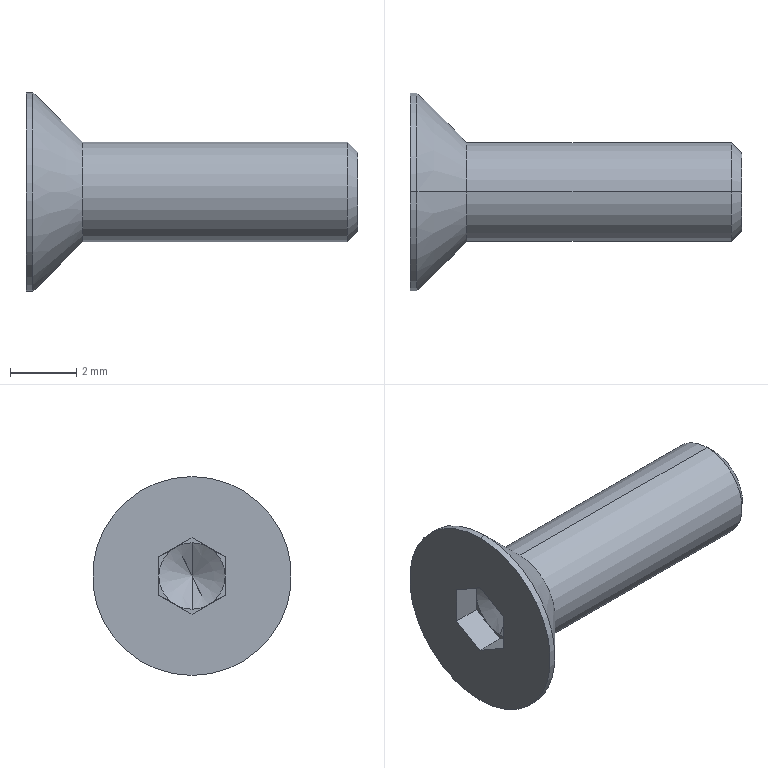Part | NX | features BREP 1 | 1 solid | 24 faces | box 10 x 6 x 6 mm | volume 85.103 mm3 | plane 14 | cone 6 | cylinder 4 | commonest cylinder face diameters 3 x2 6 x2
STEP:
#1=CARTESIAN_POINT('',(1.427,0.,0.));
#2=VERTEX_POINT('',#1);
#3=CARTESIAN_POINT('',(0.85,0.,1.));
#4=VERTEX_POINT('',#3);
#5=CARTESIAN_POINT('',(0.85,0.,1.));
#6=DIRECTION('',(-0.5,0.,0.866));
#7=VECTOR('',#6,1000.);
#8=LINE('',#5,#7);
#9=EDGE_CURVE('',#2,#4,#8,.T.);
#10=ORIENTED_EDGE('',*,*,#9,.F.);
#11=CARTESIAN_POINT('',(0.85,0.,-1.));
#12=VERTEX_POINT('',#11);
#13=CARTESIAN_POINT('',(0.85,0.,-1.));
#14=DIRECTION('',(-0.5,0.,-0.866));
#15=VECTOR('',#14,1000.);
#16=LINE('',#13,#15);
#17=EDGE_CURVE('',#2,#12,#16,.T.);
#18=ORIENTED_EDGE('',*,*,#17,.T.);
#19=CARTESIAN_POINT('',(0.85,-0.5,-0.866));
#20=VERTEX_POINT('',#19);
#21=CARTESIAN_POINT('',(0.85,0.,0.));
#22=DIRECTION('',(-1.,0.,0.));
#23=DIRECTION('',(0.,0.,1.));
#24=AXIS2_PLACEMENT_3D('',#21,#22,#23);
#25=CIRCLE('',#24,1.);
#26=EDGE_CURVE('',#12,#20,#25,.T.);
#27=ORIENTED_EDGE('',*,*,#26,.T.);
#28=CARTESIAN_POINT('',(0.85,-1.,0.));
#29=VERTEX_POINT('',#28);
#30=CARTESIAN_POINT('',(0.85,0.,0.));
#31=DIRECTION('',(-1.,0.,0.));
#32=DIRECTION('',(0.,0.,1.));
#33=AXIS2_PLACEMENT_3D('',#30,#31,#32);
#34=CIRCLE('',#33,1.);
#35=EDGE_CURVE('',#20,#29,#34,.T.);
#36=ORIENTED_EDGE('',*,*,#35,.T.);
#37=CARTESIAN_POINT('',(0.85,-0.5,0.866));
#38=VERTEX_POINT('',#37);
#39=CARTESIAN_POINT('',(0.85,0.,0.));
#40=DIRECTION('',(-1.,0.,0.));
#41=DIRECTION('',(0.,0.,1.));
#42=AXIS2_PLACEMENT_3D('',#39,#40,#41);
#43=CIRCLE('',#42,1.);
#44=EDGE_CURVE('',#29,#38,#43,.T.);
#45=ORIENTED_EDGE('',*,*,#44,.T.);
#46=CARTESIAN_POINT('',(0.85,0.,0.));
#47=DIRECTION('',(-1.,0.,0.));
#48=DIRECTION('',(0.,0.,1.));
#49=AXIS2_PLACEMENT_3D('',#46,#47,#48);
#50=CIRCLE('',#49,1.);
#51=EDGE_CURVE('',#38,#4,#50,.T.);
#52=ORIENTED_EDGE('',*,*,#51,.T.);
#53=EDGE_LOOP('',(#10,#18,#27,#36,#45,#52));
#54=FACE_BOUND('',#53,.T.);
#55=CARTESIAN_POINT('',(0.85,0.,0.));
#56=DIRECTION('',(-1.,0.,0.));
#57=DIRECTION('',(0.,0.,-1.));
#58=AXIS2_PLACEMENT_3D('',#55,#56,#57);
#59=CONICAL_SURFACE('',#58,1.,1.047);
#60=ADVANCED_FACE('',(#54),#59,.F.);
#61=CARTESIAN_POINT('',(10.,0.,1.194));
#62=VERTEX_POINT('',#61);
#63=CARTESIAN_POINT('',(10.,0.,-1.194));
#64=VERTEX_POINT('',#63);
#65=CARTESIAN_POINT('',(10.,0.,0.));
#66=DIRECTION('',(-1.,0.,0.));
#67=DIRECTION('',(0.,0.,1.));
#68=AXIS2_PLACEMENT_3D('',#65,#66,#67);
#69=CIRCLE('',#68,1.194);
#70=EDGE_CURVE('',#62,#64,#69,.T.);
#71=ORIENTED_EDGE('',*,*,#70,.T.);
#72=CARTESIAN_POINT('',(9.694,0.,-1.5));
#73=VERTEX_POINT('',#72);
#74=CARTESIAN_POINT('',(10.,0.,-1.194));
#75=DIRECTION('',(-0.7071,0.,-0.7071));
#76=VECTOR('',#75,1000.);
#77=LINE('',#74,#76);
#78=EDGE_CURVE('',#64,#73,#77,.T.);
#79=ORIENTED_EDGE('',*,*,#78,.T.);
#80=CARTESIAN_POINT('',(9.694,0.,1.5));
#81=VERTEX_POINT('',#80);
#82=CARTESIAN_POINT('',(9.694,0.,0.));
#83=DIRECTION('',(-1.,0.,0.));
#84=DIRECTION('',(0.,0.,1.));
#85=AXIS2_PLACEMENT_3D('',#82,#83,#84);
#86=CIRCLE('',#85,1.5);
#87=EDGE_CURVE('',#81,#73,#86,.T.);
#88=ORIENTED_EDGE('',*,*,#87,.F.);
#89=CARTESIAN_POINT('',(10.,0.,1.194));
#90=DIRECTION('',(-0.7071,0.,0.7071));
#91=VECTOR('',#90,1000.);
#92=LINE('',#89,#91);
#93=EDGE_CURVE('',#62,#81,#92,.T.);
#94=ORIENTED_EDGE('',*,*,#93,.F.);
#95=EDGE_LOOP('',(#71,#79,#88,#94));
#96=FACE_BOUND('',#95,.T.);
#97=CARTESIAN_POINT('',(10.,0.,0.));
#98=DIRECTION('',(-1.,0.,0.));
#99=DIRECTION('',(0.,0.,-1.));
#100=AXIS2_PLACEMENT_3D('',#97,#98,#99);
#101=CONICAL_SURFACE('',#100,1.194,0.7854);
#102=ADVANCED_FACE('',(#96),#101,.T.);
#103=ORIENTED_EDGE('',*,*,#87,.T.);
#104=CARTESIAN_POINT('',(1.7,0.,-1.5));
#105=VERTEX_POINT('',#104);
#106=CARTESIAN_POINT('',(10.,0.,-1.5));
#107=DIRECTION('',(-1.,0.,0.));
#108=VECTOR('',#107,1000.);
#109=LINE('',#106,#108);
#110=EDGE_CURVE('',#73,#105,#109,.T.);
#111=ORIENTED_EDGE('',*,*,#110,.T.);
#112=CARTESIAN_POINT('',(1.7,0.,1.5));
#113=VERTEX_POINT('',#112);
#114=CARTESIAN_POINT('',(1.7,0.,0.));
#115=DIRECTION('',(-1.,0.,0.));
#116=DIRECTION('',(0.,0.,1.));
#117=AXIS2_PLACEMENT_3D('',#114,#115,#116);
#118=CIRCLE('',#117,1.5);
#119=EDGE_CURVE('',#113,#105,#118,.T.);
#120=ORIENTED_EDGE('',*,*,#119,.F.);
#121=CARTESIAN_POINT('',(10.,0.,1.5));
#122=DIRECTION('',(-1.,0.,0.));
#123=VECTOR('',#122,1000.);
#124=LINE('',#121,#123);
#125=EDGE_CURVE('',#81,#113,#124,.T.);
#126=ORIENTED_EDGE('',*,*,#125,.F.);
#127=EDGE_LOOP('',(#103,#111,#120,#126));
#128=FACE_BOUND('',#127,.T.);
#129=CARTESIAN_POINT('',(10.,0.,0.));
#130=DIRECTION('',(-1.,0.,0.));
#131=DIRECTION('',(0.,0.,-1.));
#132=AXIS2_PLACEMENT_3D('',#129,#130,#131);
#133=CYLINDRICAL_SURFACE('',#132,1.5);
#134=ADVANCED_FACE('',(#128),#133,.T.);
#135=ORIENTED_EDGE('',*,*,#119,.T.);
#136=CARTESIAN_POINT('',(0.2,0.,-3.));
#137=VERTEX_POINT('',#136);
#138=CARTESIAN_POINT('',(1.7,0.,-1.5));
#139=DIRECTION('',(-0.7071,0.,-0.7071));
#140=VECTOR('',#139,1000.);
#141=LINE('',#138,#140);
#142=EDGE_CURVE('',#105,#137,#141,.T.);
#143=ORIENTED_EDGE('',*,*,#142,.T.);
#144=CARTESIAN_POINT('',(0.2,0.,3.));
#145=VERTEX_POINT('',#144);
#146=CARTESIAN_POINT('',(0.2,0.,0.));
#147=DIRECTION('',(-1.,0.,0.));
#148=DIRECTION('',(0.,0.,1.));
#149=AXIS2_PLACEMENT_3D('',#146,#147,#148);
#150=CIRCLE('',#149,3.);
#151=EDGE_CURVE('',#145,#137,#150,.T.);
#152=ORIENTED_EDGE('',*,*,#151,.F.);
#153=CARTESIAN_POINT('',(1.7,0.,1.5));
#154=DIRECTION('',(-0.7071,0.,0.7071));
#155=VECTOR('',#154,1000.);
#156=LINE('',#153,#155);
#157=EDGE_CURVE('',#113,#145,#156,.T.);
#158=ORIENTED_EDGE('',*,*,#157,.F.);
#159=EDGE_LOOP('',(#135,#143,#152,#158));
#160=FACE_BOUND('',#159,.T.);
#161=CARTESIAN_POINT('',(1.7,0.,0.));
#162=DIRECTION('',(-1.,0.,0.));
#163=DIRECTION('',(0.,0.,-1.));
#164=AXIS2_PLACEMENT_3D('',#161,#162,#163);
#165=CONICAL_SURFACE('',#164,1.5,0.7854);
#166=ADVANCED_FACE('',(#160),#165,.T.);
#167=ORIENTED_EDGE('',*,*,#151,.T.);
#168=CARTESIAN_POINT('',(0.,0.,-3.));
#169=VERTEX_POINT('',#168);
#170=CARTESIAN_POINT('',(10.,0.,-3.));
#171=DIRECTION('',(-1.,0.,0.));
#172=VECTOR('',#171,1000.);
#173=LINE('',#170,#172);
#174=EDGE_CURVE('',#137,#169,#173,.T.);
#175=ORIENTED_EDGE('',*,*,#174,.T.);
#176=CARTESIAN_POINT('',(0.,0.,3.));
#177=VERTEX_POINT('',#176);
#178=CARTESIAN_POINT('',(0.,0.,0.));
#179=DIRECTION('',(-1.,0.,0.));
#180=DIRECTION('',(0.,0.,1.));
#181=AXIS2_PLACEMENT_3D('',#178,#179,#180);
#182=CIRCLE('',#181,3.);
#183=EDGE_CURVE('',#177,#169,#182,.T.);
#184=ORIENTED_EDGE('',*,*,#183,.F.);
#185=CARTESIAN_POINT('',(10.,0.,3.));
#186=DIRECTION('',(-1.,0.,0.));
#187=VECTOR('',#186,1000.);
#188=LINE('',#185,#187);
#189=EDGE_CURVE('',#145,#177,#188,.T.);
#190=ORIENTED_EDGE('',*,*,#189,.F.);
#191=EDGE_LOOP('',(#167,#175,#184,#190));
#192=FACE_BOUND('',#191,.T.);
#193=CARTESIAN_POINT('',(10.,0.,0.));
#194=DIRECTION('',(-1.,0.,0.));
#195=DIRECTION('',(0.,0.,-1.));
#196=AXIS2_PLACEMENT_3D('',#193,#194,#195);
#197=CYLINDRICAL_SURFACE('',#196,3.);
#198=ADVANCED_FACE('',(#192),#197,.T.);
#199=CARTESIAN_POINT('',(0.,0.,1.155));
#200=VERTEX_POINT('',#199);
#201=CARTESIAN_POINT('',(0.,-1.,0.5774));
#202=VERTEX_POINT('',#201);
#203=CARTESIAN_POINT('',(0.,0.25,1.299));
#204=DIRECTION('',(0.,-0.866,-0.5));
#205=VECTOR('',#204,1000.);
#206=LINE('',#203,#205);
#207=EDGE_CURVE('',#200,#202,#206,.T.);
#208=ORIENTED_EDGE('',*,*,#207,.T.);
#209=CARTESIAN_POINT('',(0.,-1.,-0.5774));
#210=VERTEX_POINT('',#209);
#211=CARTESIAN_POINT('',(0.,-1.,0.));
#212=DIRECTION('',(0.,0.,-1.));
#213=VECTOR('',#212,1000.);
#214=LINE('',#211,#213);
#215=EDGE_CURVE('',#202,#210,#214,.T.);
#216=ORIENTED_EDGE('',*,*,#215,.T.);
#217=CARTESIAN_POINT('',(0.,0.,-1.155));
#218=VERTEX_POINT('',#217);
#219=CARTESIAN_POINT('',(0.,0.25,-1.299));
#220=DIRECTION('',(0.,0.866,-0.5));
#221=VECTOR('',#220,1000.);
#222=LINE('',#219,#221);
#223=EDGE_CURVE('',#210,#218,#222,.T.);
#224=ORIENTED_EDGE('',*,*,#223,.T.);
#225=CARTESIAN_POINT('',(0.,1.,-0.5774));
#226=VERTEX_POINT('',#225);
#227=CARTESIAN_POINT('',(0.,1.25,-0.433));
#228=DIRECTION('',(0.,0.866,0.5));
#229=VECTOR('',#228,1000.);
#230=LINE('',#227,#229);
#231=EDGE_CURVE('',#218,#226,#230,.T.);
#232=ORIENTED_EDGE('',*,*,#231,.T.);
#233=CARTESIAN_POINT('',(0.,1.,0.5774));
#234=VERTEX_POINT('',#233);
#235=CARTESIAN_POINT('',(0.,1.,0.));
#236=DIRECTION('',(0.,0.,1.));
#237=VECTOR('',#236,1000.);
#238=LINE('',#235,#237);
#239=EDGE_CURVE('',#226,#234,#238,.T.);
#240=ORIENTED_EDGE('',*,*,#239,.T.);
#241=CARTESIAN_POINT('',(0.,1.25,0.433));
#242=DIRECTION('',(0.,-0.866,0.5));
#243=VECTOR('',#242,1000.);
#244=LINE('',#241,#243);
#245=EDGE_CURVE('',#234,#200,#244,.T.);
#246=ORIENTED_EDGE('',*,*,#245,.T.);
#247=EDGE_LOOP('',(#208,#216,#224,#232,#240,#246));
#248=FACE_BOUND('',#247,.T.);
#249=ORIENTED_EDGE('',*,*,#183,.T.);
#250=CARTESIAN_POINT('',(0.,0.,0.));
#251=DIRECTION('',(-1.,0.,0.));
#252=DIRECTION('',(0.,0.,1.));
#253=AXIS2_PLACEMENT_3D('',#250,#251,#252);
#254=CIRCLE('',#253,3.);
#255=EDGE_CURVE('',#169,#177,#254,.T.);
#256=ORIENTED_EDGE('',*,*,#255,.T.);
#257=EDGE_LOOP('',(#249,#256));
#258=FACE_BOUND('',#257,.T.);
#259=CARTESIAN_POINT('',(0.,1.,0.));
#260=DIRECTION('',(1.,0.,0.));
#261=DIRECTION('',(0.,0.,1.));
#262=AXIS2_PLACEMENT_3D('',#259,#260,#261);
#263=PLANE('',#262);
#264=ADVANCED_FACE('',(#248,#258),#263,.F.);
#265=ORIENTED_EDGE('',*,*,#174,.F.);
#266=CARTESIAN_POINT('',(0.2,0.,0.));
#267=DIRECTION('',(-1.,0.,0.));
#268=DIRECTION('',(0.,0.,1.));
#269=AXIS2_PLACEMENT_3D('',#266,#267,#268);
#270=CIRCLE('',#269,3.);
#271=EDGE_CURVE('',#137,#145,#270,.T.);
#272=ORIENTED_EDGE('',*,*,#271,.T.);
#273=ORIENTED_EDGE('',*,*,#189,.T.);
#274=ORIENTED_EDGE('',*,*,#255,.F.);
#275=EDGE_LOOP('',(#265,#272,#273,#274));
#276=FACE_BOUND('',#275,.T.);
#277=CARTESIAN_POINT('',(10.,0.,0.));
#278=DIRECTION('',(-1.,0.,0.));
#279=DIRECTION('',(0.,0.,-1.));
#280=AXIS2_PLACEMENT_3D('',#277,#278,#279);
#281=CYLINDRICAL_SURFACE('',#280,3.);
#282=ADVANCED_FACE('',(#276),#281,.T.);
#283=ORIENTED_EDGE('',*,*,#142,.F.);
#284=CARTESIAN_POINT('',(1.7,0.,0.));
#285=DIRECTION('',(-1.,0.,0.));
#286=DIRECTION('',(0.,0.,1.));
#287=AXIS2_PLACEMENT_3D('',#284,#285,#286);
#288=CIRCLE('',#287,1.5);
#289=EDGE_CURVE('',#105,#113,#288,.T.);
#290=ORIENTED_EDGE('',*,*,#289,.T.);
#291=ORIENTED_EDGE('',*,*,#157,.T.);
#292=ORIENTED_EDGE('',*,*,#271,.F.);
#293=EDGE_LOOP('',(#283,#290,#291,#292));
#294=FACE_BOUND('',#293,.T.);
#295=CARTESIAN_POINT('',(1.7,0.,0.));
#296=DIRECTION('',(-1.,0.,0.));
#297=DIRECTION('',(0.,0.,-1.));
#298=AXIS2_PLACEMENT_3D('',#295,#296,#297);
#299=CONICAL_SURFACE('',#298,1.5,0.7854);
#300=ADVANCED_FACE('',(#294),#299,.T.);
#301=ORIENTED_EDGE('',*,*,#110,.F.);
#302=CARTESIAN_POINT('',(9.694,0.,0.));
#303=DIRECTION('',(-1.,0.,0.));
#304=DIRECTION('',(0.,0.,1.));
#305=AXIS2_PLACEMENT_3D('',#302,#303,#304);
#306=CIRCLE('',#305,1.5);
#307=EDGE_CURVE('',#73,#81,#306,.T.);
#308=ORIENTED_EDGE('',*,*,#307,.T.);
#309=ORIENTED_EDGE('',*,*,#125,.T.);
#310=ORIENTED_EDGE('',*,*,#289,.F.);
#311=EDGE_LOOP('',(#301,#308,#309,#310));
#312=FACE_BOUND('',#311,.T.);
#313=CARTESIAN_POINT('',(10.,0.,0.));
#314=DIRECTION('',(-1.,0.,0.));
#315=DIRECTION('',(0.,0.,-1.));
#316=AXIS2_PLACEMENT_3D('',#313,#314,#315);
#317=CYLINDRICAL_SURFACE('',#316,1.5);
#318=ADVANCED_FACE('',(#312),#317,.T.);
#319=ORIENTED_EDGE('',*,*,#78,.F.);
#320=CARTESIAN_POINT('',(10.,0.,0.));
#321=DIRECTION('',(-1.,0.,0.));
#322=DIRECTION('',(0.,0.,1.));
#323=AXIS2_PLACEMENT_3D('',#320,#321,#322);
#324=CIRCLE('',#323,1.194);
#325=EDGE_CURVE('',#64,#62,#324,.T.);
#326=ORIENTED_EDGE('',*,*,#325,.T.);
#327=ORIENTED_EDGE('',*,*,#93,.T.);
#328=ORIENTED_EDGE('',*,*,#307,.F.);
#329=EDGE_LOOP('',(#319,#326,#327,#328));
#330=FACE_BOUND('',#329,.T.);
#331=CARTESIAN_POINT('',(10.,0.,0.));
#332=DIRECTION('',(-1.,0.,0.));
#333=DIRECTION('',(0.,0.,-1.));
#334=AXIS2_PLACEMENT_3D('',#331,#332,#333);
#335=CONICAL_SURFACE('',#334,1.194,0.7854);
#336=ADVANCED_FACE('',(#330),#335,.T.);
#337=ORIENTED_EDGE('',*,*,#70,.F.);
#338=ORIENTED_EDGE('',*,*,#325,.F.);
#339=EDGE_LOOP('',(#337,#338));
#340=FACE_BOUND('',#339,.T.);
#341=CARTESIAN_POINT('',(10.,1.194,0.));
#342=DIRECTION('',(-1.,0.,0.));
#343=DIRECTION('',(0.,0.,-1.));
#344=AXIS2_PLACEMENT_3D('',#341,#342,#343);
#345=PLANE('',#344);
#346=ADVANCED_FACE('',(#340),#345,.F.);
#347=ORIENTED_EDGE('',*,*,#44,.F.);
#348=CARTESIAN_POINT('',(0.85,-1.,0.5774));
#349=VERTEX_POINT('',#348);
#350=CARTESIAN_POINT('',(0.85,-1.,-0.5774));
#351=DIRECTION('',(0.,0.,1.));
#352=VECTOR('',#351,1000.);
#353=LINE('',#350,#352);
#354=EDGE_CURVE('',#29,#349,#353,.T.);
#355=ORIENTED_EDGE('',*,*,#354,.T.);
#356=CARTESIAN_POINT('',(0.85,-1.,0.5774));
#357=DIRECTION('',(0.,0.866,0.5));
#358=VECTOR('',#357,1000.);
#359=LINE('',#356,#358);
#360=EDGE_CURVE('',#349,#38,#359,.T.);
#361=ORIENTED_EDGE('',*,*,#360,.T.);
#362=EDGE_LOOP('',(#347,#355,#361));
#363=FACE_BOUND('',#362,.T.);
#364=CARTESIAN_POINT('',(0.85,0.,0.));
#365=DIRECTION('',(-1.,0.,0.));
#366=DIRECTION('',(0.,0.,-1.));
#367=AXIS2_PLACEMENT_3D('',#364,#365,#366);
#368=PLANE('',#367);
#369=ADVANCED_FACE('',(#363),#368,.T.);
#370=ORIENTED_EDGE('',*,*,#35,.F.);
#371=CARTESIAN_POINT('',(0.85,-1.,-0.5774));
#372=VERTEX_POINT('',#371);
#373=CARTESIAN_POINT('',(0.85,0.,-1.155));
#374=DIRECTION('',(0.,-0.866,0.5));
#375=VECTOR('',#374,1000.);
#376=LINE('',#373,#375);
#377=EDGE_CURVE('',#20,#372,#376,.T.);
#378=ORIENTED_EDGE('',*,*,#377,.T.);
#379=CARTESIAN_POINT('',(0.85,-1.,-0.5774));
#380=DIRECTION('',(0.,0.,1.));
#381=VECTOR('',#380,1000.);
#382=LINE('',#379,#381);
#383=EDGE_CURVE('',#372,#29,#382,.T.);
#384=ORIENTED_EDGE('',*,*,#383,.T.);
#385=EDGE_LOOP('',(#370,#378,#384));
#386=FACE_BOUND('',#385,.T.);
#387=CARTESIAN_POINT('',(0.85,0.,0.));
#388=DIRECTION('',(-1.,0.,0.));
#389=DIRECTION('',(0.,0.,-1.));
#390=AXIS2_PLACEMENT_3D('',#387,#388,#389);
#391=PLANE('',#390);
#392=ADVANCED_FACE('',(#386),#391,.T.);
#393=CARTESIAN_POINT('',(0.85,0.5,-0.866));
#394=VERTEX_POINT('',#393);
#395=CARTESIAN_POINT('',(0.85,0.,0.));
#396=DIRECTION('',(-1.,0.,0.));
#397=DIRECTION('',(0.,0.,1.));
#398=AXIS2_PLACEMENT_3D('',#395,#396,#397);
#399=CIRCLE('',#398,1.);
#400=EDGE_CURVE('',#394,#12,#399,.T.);
#401=ORIENTED_EDGE('',*,*,#400,.F.);
#402=CARTESIAN_POINT('',(0.85,0.,-1.155));
#403=VERTEX_POINT('',#402);
#404=CARTESIAN_POINT('',(0.85,1.,-0.5774));
#405=DIRECTION('',(0.,-0.866,-0.5));
#406=VECTOR('',#405,1000.);
#407=LINE('',#404,#406);
#408=EDGE_CURVE('',#394,#403,#407,.T.);
#409=ORIENTED_EDGE('',*,*,#408,.T.);
#410=CARTESIAN_POINT('',(0.85,0.,-1.155));
#411=DIRECTION('',(0.,-0.866,0.5));
#412=VECTOR('',#411,1000.);
#413=LINE('',#410,#412);
#414=EDGE_CURVE('',#403,#20,#413,.T.);
#415=ORIENTED_EDGE('',*,*,#414,.T.);
#416=ORIENTED_EDGE('',*,*,#26,.F.);
#417=EDGE_LOOP('',(#401,#409,#415,#416));
#418=FACE_BOUND('',#417,.T.);
#419=CARTESIAN_POINT('',(0.85,0.,0.));
#420=DIRECTION('',(-1.,0.,0.));
#421=DIRECTION('',(0.,0.,-1.));
#422=AXIS2_PLACEMENT_3D('',#419,#420,#421);
#423=PLANE('',#422);
#424=ADVANCED_FACE('',(#418),#423,.T.);
#425=CARTESIAN_POINT('',(0.85,1.,0.));
#426=VERTEX_POINT('',#425);
#427=CARTESIAN_POINT('',(0.85,0.,0.));
#428=DIRECTION('',(-1.,0.,0.));
#429=DIRECTION('',(0.,0.,1.));
#430=AXIS2_PLACEMENT_3D('',#427,#428,#429);
#431=CIRCLE('',#430,1.);
#432=EDGE_CURVE('',#426,#394,#431,.T.);
#433=ORIENTED_EDGE('',*,*,#432,.F.);
#434=CARTESIAN_POINT('',(0.85,1.,-0.5774));
#435=VERTEX_POINT('',#434);
#436=CARTESIAN_POINT('',(0.85,1.,0.5774));
#437=DIRECTION('',(0.,0.,-1.));
#438=VECTOR('',#437,1000.);
#439=LINE('',#436,#438);
#440=EDGE_CURVE('',#426,#435,#439,.T.);
#441=ORIENTED_EDGE('',*,*,#440,.T.);
#442=CARTESIAN_POINT('',(0.85,1.,-0.5774));
#443=DIRECTION('',(0.,-0.866,-0.5));
#444=VECTOR('',#443,1000.);
#445=LINE('',#442,#444);
#446=EDGE_CURVE('',#435,#394,#445,.T.);
#447=ORIENTED_EDGE('',*,*,#446,.T.);
#448=EDGE_LOOP('',(#433,#441,#447));
#449=FACE_BOUND('',#448,.T.);
#450=CARTESIAN_POINT('',(0.85,0.,0.));
#451=DIRECTION('',(-1.,0.,0.));
#452=DIRECTION('',(0.,0.,-1.));
#453=AXIS2_PLACEMENT_3D('',#450,#451,#452);
#454=PLANE('',#453);
#455=ADVANCED_FACE('',(#449),#454,.T.);
#456=CARTESIAN_POINT('',(0.85,0.5,0.866));
#457=VERTEX_POINT('',#456);
#458=CARTESIAN_POINT('',(0.85,0.,0.));
#459=DIRECTION('',(-1.,0.,0.));
#460=DIRECTION('',(0.,0.,1.));
#461=AXIS2_PLACEMENT_3D('',#458,#459,#460);
#462=CIRCLE('',#461,1.);
#463=EDGE_CURVE('',#457,#426,#462,.T.);
#464=ORIENTED_EDGE('',*,*,#463,.F.);
#465=CARTESIAN_POINT('',(0.85,1.,0.5774));
#466=VERTEX_POINT('',#465);
#467=CARTESIAN_POINT('',(0.85,0.,1.155));
#468=DIRECTION('',(0.,0.866,-0.5));
#469=VECTOR('',#468,1000.);
#470=LINE('',#467,#469);
#471=EDGE_CURVE('',#457,#466,#470,.T.);
#472=ORIENTED_EDGE('',*,*,#471,.T.);
#473=CARTESIAN_POINT('',(0.85,1.,0.5774));
#474=DIRECTION('',(0.,0.,-1.));
#475=VECTOR('',#474,1000.);
#476=LINE('',#473,#475);
#477=EDGE_CURVE('',#466,#426,#476,.T.);
#478=ORIENTED_EDGE('',*,*,#477,.T.);
#479=EDGE_LOOP('',(#464,#472,#478));
#480=FACE_BOUND('',#479,.T.);
#481=CARTESIAN_POINT('',(0.85,0.,0.));
#482=DIRECTION('',(-1.,0.,0.));
#483=DIRECTION('',(0.,0.,-1.));
#484=AXIS2_PLACEMENT_3D('',#481,#482,#483);
#485=PLANE('',#484);
#486=ADVANCED_FACE('',(#480),#485,.T.);
#487=ORIENTED_EDGE('',*,*,#51,.F.);
#488=CARTESIAN_POINT('',(0.85,0.,1.155));
#489=VERTEX_POINT('',#488);
#490=CARTESIAN_POINT('',(0.85,-1.,0.5774));
#491=DIRECTION('',(0.,0.866,0.5));
#492=VECTOR('',#491,1000.);
#493=LINE('',#490,#492);
#494=EDGE_CURVE('',#38,#489,#493,.T.);
#495=ORIENTED_EDGE('',*,*,#494,.T.);
#496=CARTESIAN_POINT('',(0.85,0.,1.155));
#497=DIRECTION('',(0.,0.866,-0.5));
#498=VECTOR('',#497,1000.);
#499=LINE('',#496,#498);
#500=EDGE_CURVE('',#489,#457,#499,.T.);
#501=ORIENTED_EDGE('',*,*,#500,.T.);
#502=CARTESIAN_POINT('',(0.85,0.,0.));
#503=DIRECTION('',(-1.,0.,0.));
#504=DIRECTION('',(0.,0.,1.));
#505=AXIS2_PLACEMENT_3D('',#502,#503,#504);
#506=CIRCLE('',#505,1.);
#507=EDGE_CURVE('',#4,#457,#506,.T.);
#508=ORIENTED_EDGE('',*,*,#507,.F.);
#509=EDGE_LOOP('',(#487,#495,#501,#508));
#510=FACE_BOUND('',#509,.T.);
#511=CARTESIAN_POINT('',(0.85,0.,0.));
#512=DIRECTION('',(-1.,0.,0.));
#513=DIRECTION('',(0.,0.,-1.));
#514=AXIS2_PLACEMENT_3D('',#511,#512,#513);
#515=PLANE('',#514);
#516=ADVANCED_FACE('',(#510),#515,.T.);
#517=ORIENTED_EDGE('',*,*,#215,.F.);
#518=CARTESIAN_POINT('',(0.85,-1.,0.5774));
#519=DIRECTION('',(-1.,0.,0.));
#520=VECTOR('',#519,1000.);
#521=LINE('',#518,#520);
#522=EDGE_CURVE('',#349,#202,#521,.T.);
#523=ORIENTED_EDGE('',*,*,#522,.F.);
#524=ORIENTED_EDGE('',*,*,#354,.F.);
#525=ORIENTED_EDGE('',*,*,#383,.F.);
#526=CARTESIAN_POINT('',(0.85,-1.,-0.5774));
#527=DIRECTION('',(-1.,0.,0.));
#528=VECTOR('',#527,1000.);
#529=LINE('',#526,#528);
#530=EDGE_CURVE('',#372,#210,#529,.T.);
#531=ORIENTED_EDGE('',*,*,#530,.T.);
#532=EDGE_LOOP('',(#517,#523,#524,#525,#531));
#533=FACE_BOUND('',#532,.T.);
#534=CARTESIAN_POINT('',(0.85,-1.,-0.5774));
#535=DIRECTION('',(0.,-1.,0.));
#536=DIRECTION('',(0.,0.,1.));
#537=AXIS2_PLACEMENT_3D('',#534,#535,#536);
#538=PLANE('',#537);
#539=ADVANCED_FACE('',(#533),#538,.F.);
#540=ORIENTED_EDGE('',*,*,#223,.F.);
#541=ORIENTED_EDGE('',*,*,#530,.F.);
#542=ORIENTED_EDGE('',*,*,#377,.F.);
#543=ORIENTED_EDGE('',*,*,#414,.F.);
#544=CARTESIAN_POINT('',(0.85,0.,-1.155));
#545=DIRECTION('',(-1.,0.,0.));
#546=VECTOR('',#545,1000.);
#547=LINE('',#544,#546);
#548=EDGE_CURVE('',#403,#218,#547,.T.);
#549=ORIENTED_EDGE('',*,*,#548,.T.);
#550=EDGE_LOOP('',(#540,#541,#542,#543,#549));
#551=FACE_BOUND('',#550,.T.);
#552=CARTESIAN_POINT('',(0.85,0.,-1.155));
#553=DIRECTION('',(0.,-0.5,-0.866));
#554=DIRECTION('',(0.,-0.866,0.5));
#555=AXIS2_PLACEMENT_3D('',#552,#553,#554);
#556=PLANE('',#555);
#557=ADVANCED_FACE('',(#551),#556,.F.);
#558=ORIENTED_EDGE('',*,*,#231,.F.);
#559=ORIENTED_EDGE('',*,*,#548,.F.);
#560=ORIENTED_EDGE('',*,*,#408,.F.);
#561=ORIENTED_EDGE('',*,*,#446,.F.);
#562=CARTESIAN_POINT('',(0.85,1.,-0.5774));
#563=DIRECTION('',(-1.,0.,0.));
#564=VECTOR('',#563,1000.);
#565=LINE('',#562,#564);
#566=EDGE_CURVE('',#435,#226,#565,.T.);
#567=ORIENTED_EDGE('',*,*,#566,.T.);
#568=EDGE_LOOP('',(#558,#559,#560,#561,#567));
#569=FACE_BOUND('',#568,.T.);
#570=CARTESIAN_POINT('',(0.85,1.,-0.5774));
#571=DIRECTION('',(0.,0.5,-0.866));
#572=DIRECTION('',(0.,-0.866,-0.5));
#573=AXIS2_PLACEMENT_3D('',#570,#571,#572);
#574=PLANE('',#573);
#575=ADVANCED_FACE('',(#569),#574,.F.);
#576=ORIENTED_EDGE('',*,*,#239,.F.);
#577=ORIENTED_EDGE('',*,*,#566,.F.);
#578=ORIENTED_EDGE('',*,*,#440,.F.);
#579=ORIENTED_EDGE('',*,*,#477,.F.);
#580=CARTESIAN_POINT('',(0.85,1.,0.5774));
#581=DIRECTION('',(-1.,0.,0.));
#582=VECTOR('',#581,1000.);
#583=LINE('',#580,#582);
#584=EDGE_CURVE('',#466,#234,#583,.T.);
#585=ORIENTED_EDGE('',*,*,#584,.T.);
#586=EDGE_LOOP('',(#576,#577,#578,#579,#585));
#587=FACE_BOUND('',#586,.T.);
#588=CARTESIAN_POINT('',(0.85,1.,0.5774));
#589=DIRECTION('',(0.,1.,0.));
#590=DIRECTION('',(0.,0.,-1.));
#591=AXIS2_PLACEMENT_3D('',#588,#589,#590);
#592=PLANE('',#591);
#593=ADVANCED_FACE('',(#587),#592,.F.);
#594=ORIENTED_EDGE('',*,*,#245,.F.);
#595=ORIENTED_EDGE('',*,*,#584,.F.);
#596=ORIENTED_EDGE('',*,*,#471,.F.);
#597=ORIENTED_EDGE('',*,*,#500,.F.);
#598=CARTESIAN_POINT('',(0.85,0.,1.155));
#599=DIRECTION('',(-1.,0.,0.));
#600=VECTOR('',#599,1000.);
#601=LINE('',#598,#600);
#602=EDGE_CURVE('',#489,#200,#601,.T.);
#603=ORIENTED_EDGE('',*,*,#602,.T.);
#604=EDGE_LOOP('',(#594,#595,#596,#597,#603));
#605=FACE_BOUND('',#604,.T.);
#606=CARTESIAN_POINT('',(0.85,0.,1.155));
#607=DIRECTION('',(0.,0.5,0.866));
#608=DIRECTION('',(0.,0.866,-0.5));
#609=AXIS2_PLACEMENT_3D('',#606,#607,#608);
#610=PLANE('',#609);
#611=ADVANCED_FACE('',(#605),#610,.F.);
#612=ORIENTED_EDGE('',*,*,#207,.F.);
#613=ORIENTED_EDGE('',*,*,#602,.F.);
#614=ORIENTED_EDGE('',*,*,#494,.F.);
#615=ORIENTED_EDGE('',*,*,#360,.F.);
#616=ORIENTED_EDGE('',*,*,#522,.T.);
#617=EDGE_LOOP('',(#612,#613,#614,#615,#616));
#618=FACE_BOUND('',#617,.T.);
#619=CARTESIAN_POINT('',(0.85,-1.,0.5774));
#620=DIRECTION('',(0.,-0.5,0.866));
#621=DIRECTION('',(0.,0.866,0.5));
#622=AXIS2_PLACEMENT_3D('',#619,#620,#621);
#623=PLANE('',#622);
#624=ADVANCED_FACE('',(#618),#623,.F.);
#625=ORIENTED_EDGE('',*,*,#17,.F.);
#626=ORIENTED_EDGE('',*,*,#9,.T.);
#627=ORIENTED_EDGE('',*,*,#507,.T.);
#628=ORIENTED_EDGE('',*,*,#463,.T.);
#629=ORIENTED_EDGE('',*,*,#432,.T.);
#630=ORIENTED_EDGE('',*,*,#400,.T.);
#631=EDGE_LOOP('',(#625,#626,#627,#628,#629,#630));
#632=FACE_BOUND('',#631,.T.);
#633=CARTESIAN_POINT('',(0.85,0.,0.));
#634=DIRECTION('',(-1.,0.,0.));
#635=DIRECTION('',(0.,0.,-1.));
#636=AXIS2_PLACEMENT_3D('',#633,#634,#635);
#637=CONICAL_SURFACE('',#636,1.,1.047);
#638=ADVANCED_FACE('',(#632),#637,.F.);
#639=CLOSED_SHELL('',(#60,#102,#134,#166,#198,#264,#282,#300,#318,#336,#346,#369,#392,#424,#455,#486,#516,#539,#557,#575,#593,#611,#624,#638));
#640=MANIFOLD_SOLID_BREP('',#639);
#641=(LENGTH_UNIT()NAMED_UNIT(*)SI_UNIT(.MILLI.,.METRE.));
#642=UNCERTAINTY_MEASURE_WITH_UNIT(LENGTH_MEASURE(0.00001),#641,'','');
#643=(NAMED_UNIT(*)PLANE_ANGLE_UNIT()SI_UNIT($,.RADIAN.));
#644=(NAMED_UNIT(*)SI_UNIT($,.STERADIAN.)SOLID_ANGLE_UNIT());
#645=(GEOMETRIC_REPRESENTATION_CONTEXT(3)GLOBAL_UNCERTAINTY_ASSIGNED_CONTEXT((#642))GLOBAL_UNIT_ASSIGNED_CONTEXT((#641,#643,#644))REPRESENTATION_CONTEXT('',''));
#646=ADVANCED_BREP_SHAPE_REPRESENTATION('',(#640),#645);